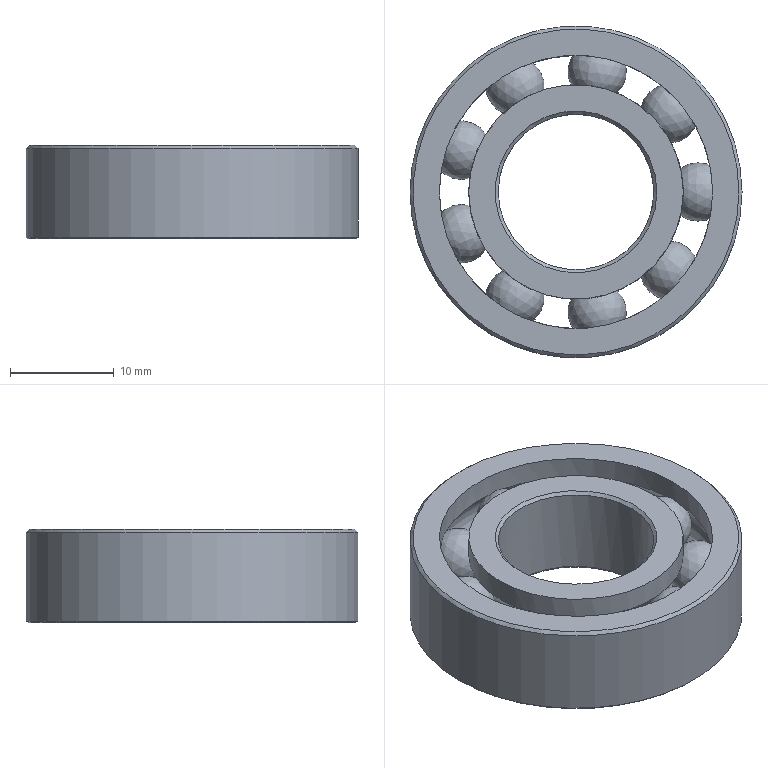Part | STEP file | YBQDJ-YL-16 | 1 solid | 41 faces | box 32 x 32 x 9 mm | volume 3911 mm3 | torus 18 | sphere 9 | cylinder 5 | cone 5 | plane 4 | commonest cylinder face diameters 20.667 x2 15 x1 26.333 x1 32 x1